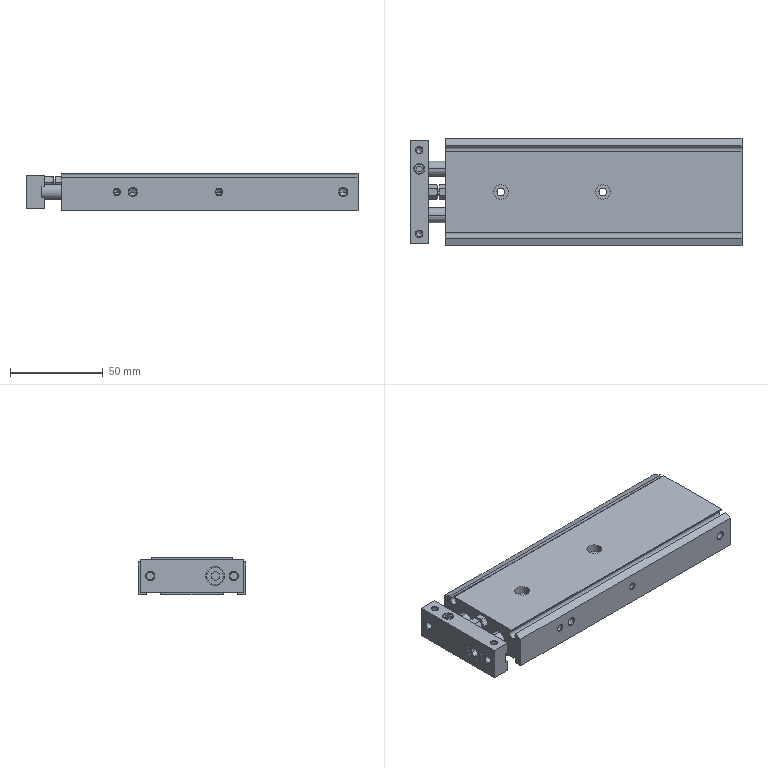Part | SolidWorks | features AEMSimFeature 1 | 2 solids | 229 faces | box 179 x 58 x 20 mm | volume 151640 mm3 | cone 84 | plane 79 | cylinder 66 | commonest cylinder face diameters 3.242 x16 4.134 x12 8 x12 16 x8 4.3 x4 4 x2